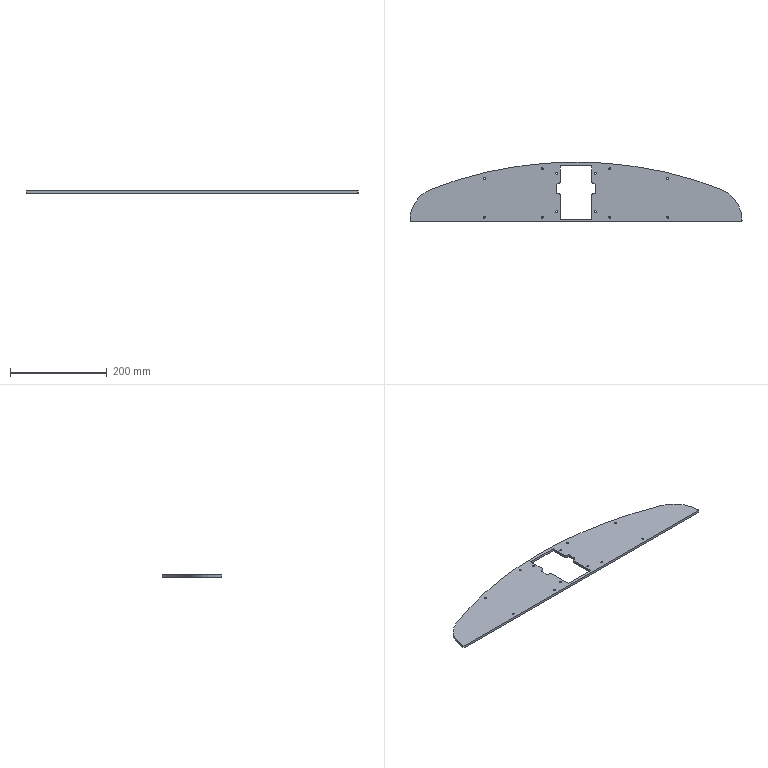Part | SolidWorks | features HoleWzd 2, ICE 2, Fillet 1, FlatPattern 1, SMBaseFlange 1, SheetMetal 1 | 1 solid | 51 faces | box 688.178 x 124 x 5 mm | volume 300076 mm3 | cylinder 36 | plane 15 | commonest cylinder face diameters 4.2 x24 6 x8 138.091 x3 1660 x1